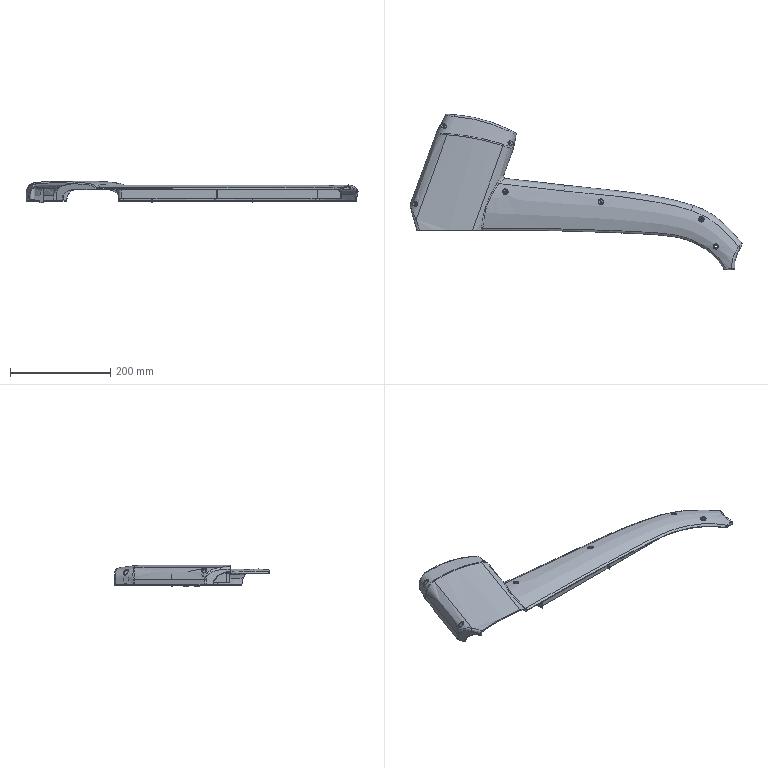Part | STEP file | PR12S0312~665.310.45RL | 1 solid | 275 faces | box 660.94 x 308.881 x 43 mm | volume 302873 mm3 | spline 112 | plane 95 | cylinder 65 | torus 3 | commonest cylinder face diameters 12 x12 8 x9 3.2 x6 8.5 x4 2 x3 5 x3